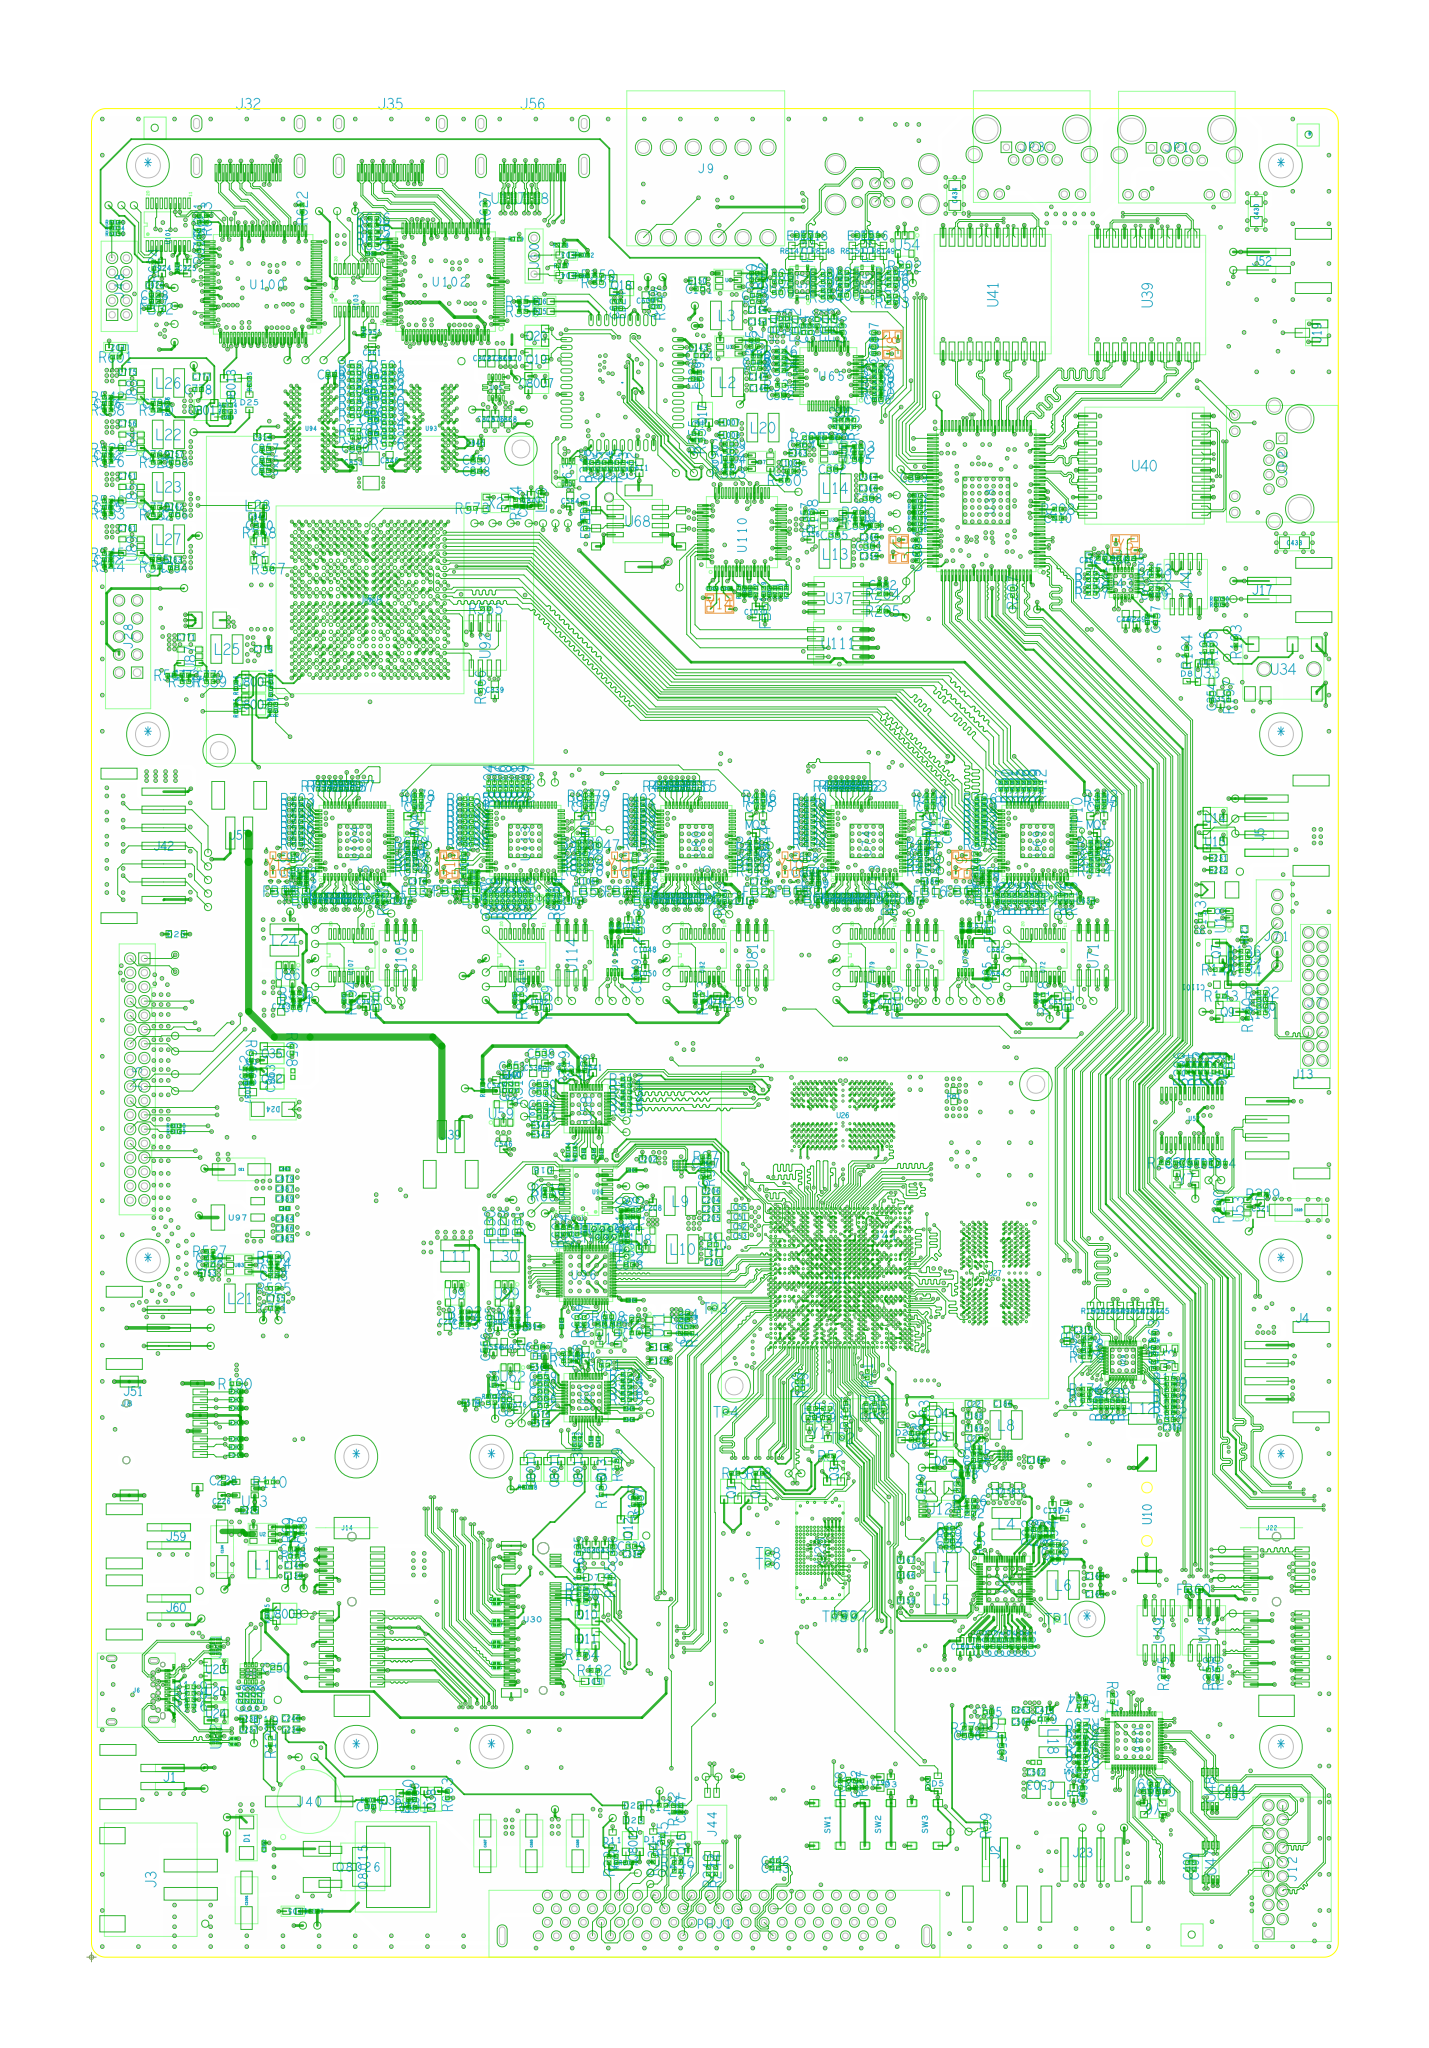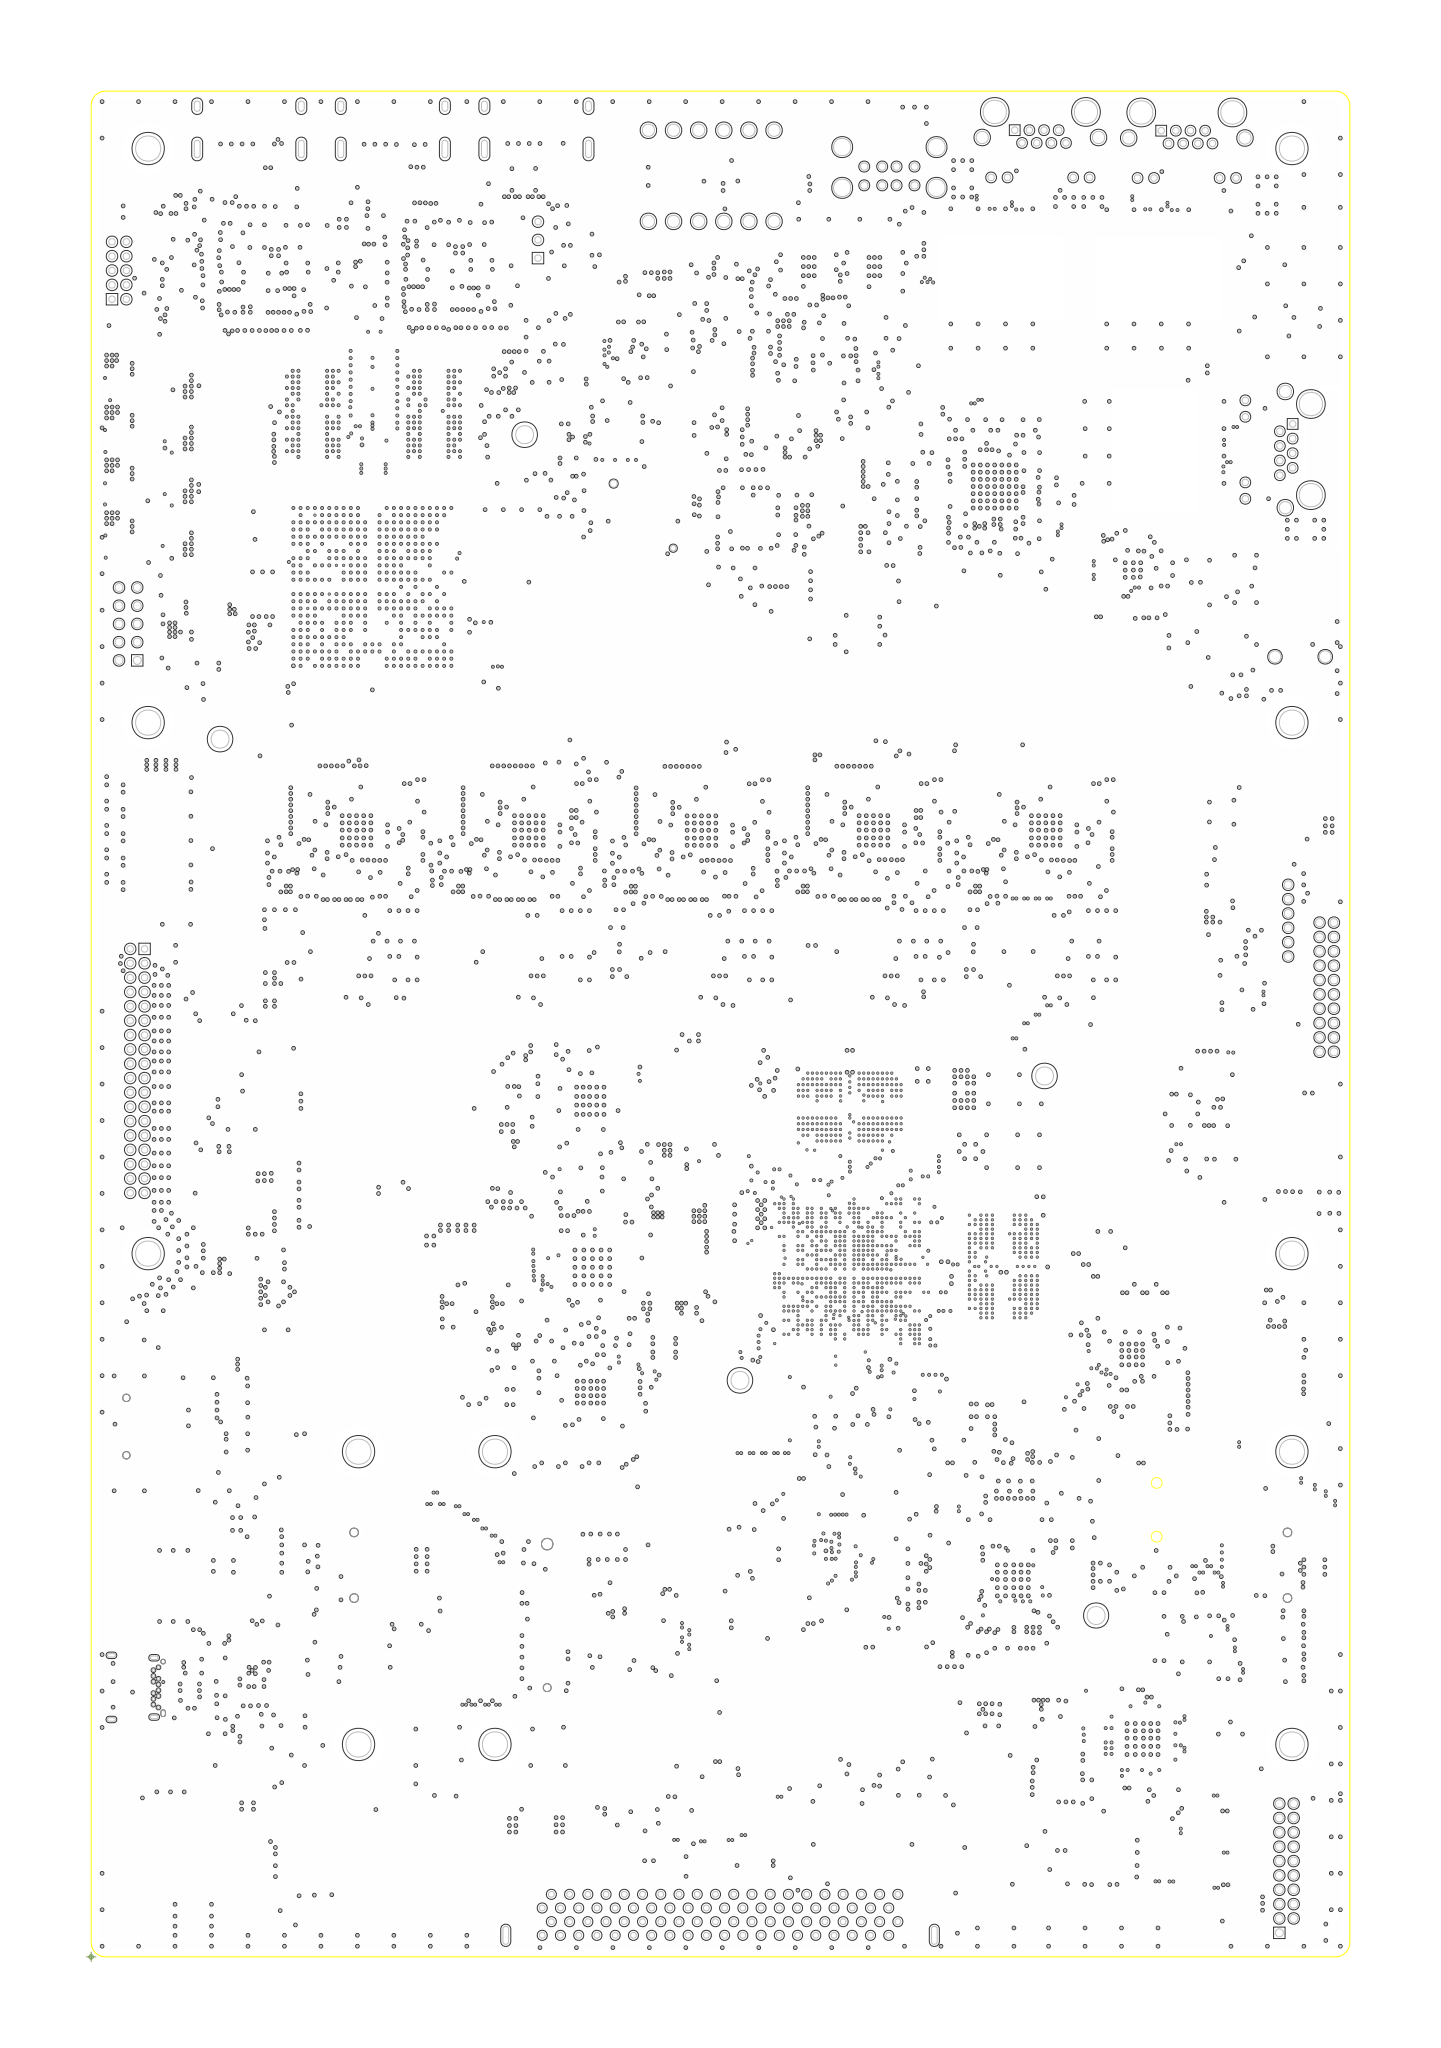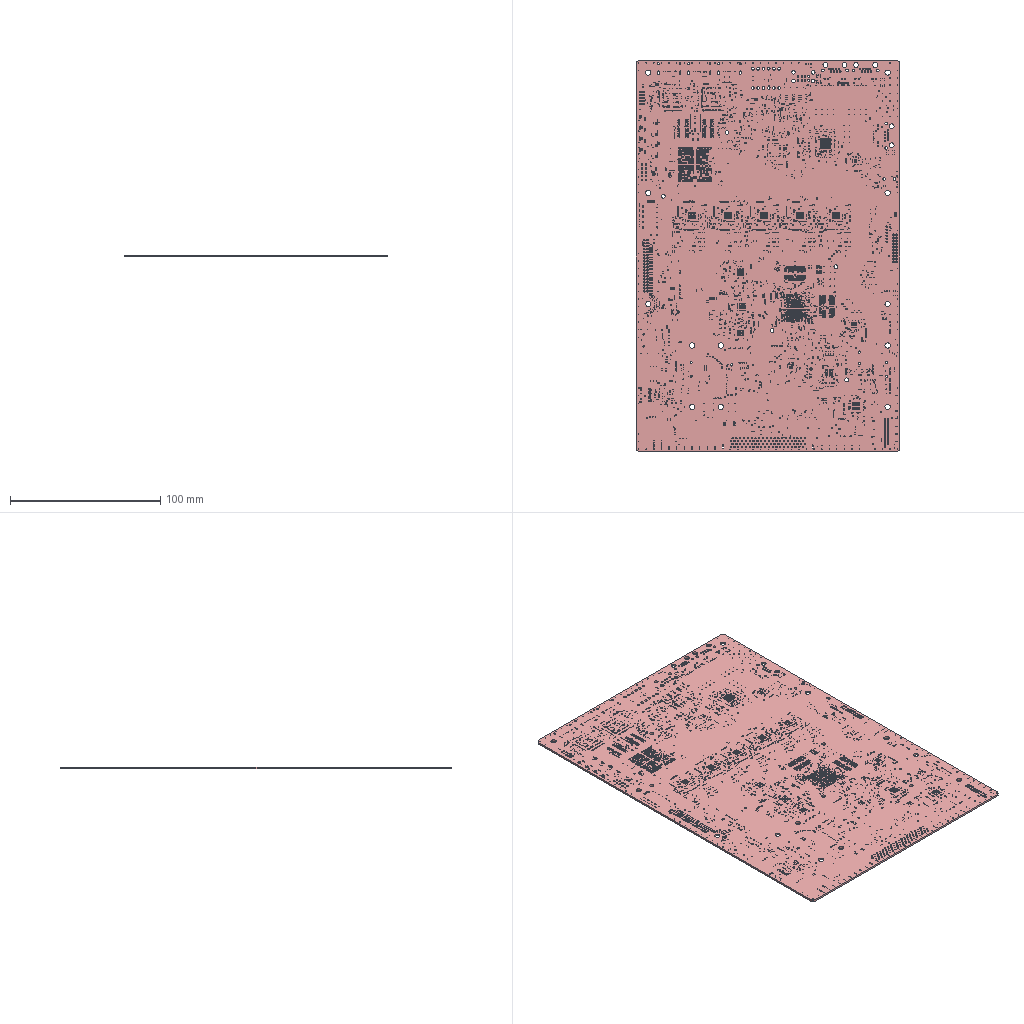Circuit board layout | Cadence Allegro | box 175.3 x 260 x 1.3 mm
Layer stack:
# Cadence Allegro layer stack of  (unit mm; from the constraint file cross-section; dielectric type: 0 not recorded (Allegro does not mark core vs prepreg), 3 surface material)
index,name,kind,layer,copper_thickness_mm,dielectric_type,dielectric_thickness_mm,dielectric_material,dielectric_constant
0,Top Surface,other,,,,,,
1,Dielectric1,dielectric,,,3,0.0249,FR-4,3.5
2,TOP,copper,TOP,0.0351,,,,
3,Dielectric2,dielectric,,,0,0.0749,FR-4,3.8
4,L2-GND,copper,L2-GND,0.017,,,,
5,Dielectric3,dielectric,,,0,0.2032,FR-4,4.5
6,L3,copper,L3,0.0305,,,,
7,Dielectric4,dielectric,,,0,0.2032,FR-4,4.5
8,L4-POWER,copper,L4-POWER,0.0305,,,,
9,Dielectric5,dielectric,,,0,0.1151,FR-4,3.8
10,L5-POWRE,copper,L5-POWRE,0.017,,,,
11,Dielectric6,dielectric,,,0,0.2032,FR-4,4.5
12,L6,copper,L6,0.0305,,,,
13,Dielectric7,dielectric,,,0,0.2032,FR-4,4.5
14,L7-GND,copper,L7-GND,0.0305,,,,
15,Dielectric8,dielectric,,,0,0.1151,FR-4,3.8
16,BOTTOM,copper,BOTTOM,0.0351,,,,
17,Dielectric9,dielectric,,,3,0.0249,FR-4,3.5
18,Bottom Surface,other,,,,,,
# drill layer pairs: low layer,high layer
drill_pair,TOP,BOTTOM
Part placement, first 572 of 2520 lines:
REFDES,COMP_VALUE,SYM_NAME,SYM_X,SYM_Y,SYM_ROTATE,SYM_MIRROR
C1,10uF,C0402,4153.838,3620.000,270.000,YES
C2,10uF,C0402,4352.539,3617.992,180.000,YES
C3,10uF,C0402,4150.000,3750.000,180.000,YES
C4,10uF,C0402,4155.807,3838.504,90.000,YES
C5,10uF,C0402,4345.767,3748.937,0.000,YES
C6,22uF,C0603,3440.000,3990.000,0.000,NO
C7,10uF,C0603,3445.000,3900.000,0.000,NO
C8,1uF,C0402,4010.744,3646.504,0.000,YES
C9,100nF,C0201,4077.744,3607.504,0.000,YES
C10,100nF,C0201,4077.744,3735.504,0.000,YES
C11,100nF,C0201,4075.497,3570.863,90.000,YES
C12,100nF,C0201,4077.744,3710.504,0.000,YES
C13,1nF,C0201,4077.744,3684.504,0.000,YES
C14,22uF,C0603,5554.744,2108.504,180.000,YES
C15,22uF,C0603,5554.744,2013.504,180.000,YES
C16,1uF,C0402,4158.744,3695.504,270.000,YES
C17,100nF,C0201,4108.744,3636.504,0.000,YES
C18,100nF,C0201,4111.744,3670.504,270.000,YES
C19,100nF,C0201,4209.744,3630.504,180.000,YES
C20,100nF,C0201,4206.744,3663.504,180.000,YES
C21,1nF,C0201,4195.744,3589.504,90.000,YES
C22,22uF,C0603,4884.744,3063.504,180.000,NO
C23,22uF,C0603,4884.744,2873.504,180.000,NO
C24,22uF,C0603,4884.744,2873.504,0.000,YES
C25,1uF,C0402,4514.744,3513.504,180.000,YES
C26,100nF,C0201,4272.744,3667.504,90.000,YES
C27,100nF,C0201,4285.744,3701.504,180.000,YES
C28,100nF,C0201,4259.744,3594.504,180.000,YES
C29,100nF,C0201,4246.744,3641.504,90.000,YES
C30,100nF,C0201,4297.744,3616.504,90.000,YES
C31,1nF,C0201,4297.744,3667.504,90.000,YES
C32,22uF,C0603,4443.208,3760.748,180.000,YES
C33,10uF,C0603,5130.000,2580.000,90.000,NO
C34,1uF,C0402,4250.000,3750.000,0.000,YES
C35,100nF,C0201,4262.744,3812.504,180.000,YES
C36,100nF,C0201,4211.744,3838.504,180.000,YES
C37,100nF,C0201,4211.744,3812.504,180.000,YES
C38,100nF,C0201,4262.744,3863.504,180.000,YES
C39,1nF,C0201,4211.744,3889.504,0.000,YES
C40,22uF,C0603,3588.681,4047.126,0.000,YES
C41,22uF,C0603,3588.681,3993.937,0.000,YES
C42,22uF,C0603,3589.744,4100.315,0.000,YES
C43,1uF,C0402,4154.822,3915.275,270.000,YES
C44,100nF,C0201,4051.744,3838.504,0.000,YES
C45,100nF,C0201,4103.744,3812.504,180.000,YES
C46,100nF,C0201,4103.744,3785.504,180.000,YES
C47,100nF,C0201,4051.744,3786.504,0.000,YES
C48,100nF,C0201,4081.744,3876.504,180.000,YES
C49,100nF,C0201,4051.744,3811.504,0.000,YES
C50,1nF,C0201,4077.744,3760.504,0.000,YES
C51,22uF,C0603,3589.744,4100.315,180.000,NO
C52,22uF,C0603,3588.681,4047.126,180.000,NO
C53,22uF,C0603,3588.681,3993.937,180.000,NO
C54,22uF,C0603,3589.744,4153.504,0.000,YES
C55,22uF,C0603,3589.744,4153.504,180.000,NO
C56,100nF,C0201,4109.744,3393.504,180.000,YES
C57,DNP,C0402,4174.744,3048.504,90.000,NO
C58,22pF,C0402,3984.744,2988.504,180.000,NO
C59,22pF,C0402,4064.744,2988.504,180.000,NO
C60,100nF,C0201,4387.539,3827.992,180.000,YES
C61,100nF,C0201,4052.539,3517.992,90.000,YES
C62,1uF,C0402,3977.539,3522.992,90.000,YES
C63,100nF,C0201,3947.539,3877.992,0.000,YES
C64,100nF,C0201,4362.539,3672.992,180.000,YES
C65,100nF,C0201,3912.539,3552.992,0.000,YES
C66,22uF,C0603,4678.744,3748.504,270.000,YES
C67,10uF,C0402,4378.646,3980.311,180.000,YES
C68,1uF,C0402,4091.744,4005.504,0.000,YES
C69,100nF,C0201,4118.539,3956.992,270.000,YES
C70,100nF,C0201,4226.744,3978.504,270.000,YES
C71,100nF,C0201,4093.539,3956.992,270.000,YES
C72,100nF,C0201,4201.744,3978.504,270.000,YES
C73,100nF,C0201,4272.744,3956.504,270.000,YES
C74,100nF,C0201,4145.744,3976.504,270.000,YES
C75,22uF,C0603,4159.744,4424.504,90.000,YES
C76,10uF,C0402,4432.539,3673.992,180.000,YES
C77,1uF,C0402,5202.744,4143.504,180.000,YES
C78,100nF,C0201,4288.539,3888.992,0.000,YES
C79,100nF,C0201,4339.744,3786.504,180.000,YES
C80,100nF,C0201,4312.744,3922.504,180.000,YES
C81,100nF,C0201,4336.744,3875.504,180.000,YES
C82,100nF,C0201,4338.744,3850.504,180.000,YES
C83,100nF,C0201,4309.744,3825.504,0.000,YES
C84,100nF,C0201,4297.744,3956.504,270.000,YES
C85,100nF,C0201,4232.744,4017.504,0.000,YES
C86,100nF,C0201,4148.744,3525.504,180.000,YES
C87,100nF,C0201,4340.744,3710.504,180.000,YES
C88,100nF,C0201,4390.744,3854.504,180.000,YES
C89,100nF,C0201,4169.539,3980.992,270.000,YES
C90,100nF,C0201,4386.520,3645.666,180.000,YES
C91,100nF,C0201,3990.539,3956.992,90.000,YES
C92,100nF,C0201,4155.744,3559.504,90.000,YES
C93,100nF,C0201,4137.744,3491.504,90.000,YES
C94,100nF,C0201,4099.119,3570.863,270.000,YES
C95,100nF,C0201,4077.744,3483.504,0.000,YES
C96,100nF,C0201,3957.000,3701.000,270.000,YES
C97,100nF,C0201,4209.355,3716.532,180.000,YES
C98,100nF,C0201,4204.744,3687.504,0.000,YES
C99,100nF,C0201,3916.744,3622.504,270.000,YES
C100,100nF,C0201,3812.744,3434.504,90.000,YES
C101,100nF,C0201,4209.744,3546.504,270.000,YES
C102,10nF,C0402,4229.586,958.561,270.000,NO
C103,100nF,C0201,3947.539,3827.992,0.000,YES
C104,100nF,C0201,4364.744,3523.504,180.000,YES
C105,100nF,C0201,3922.539,3927.992,0.000,YES
C106,100nF,C0201,3945.576,3799.209,0.000,YES
C107,100nF,C0201,4704.744,3378.504,180.000,YES
C108,100nF,C0201,4704.744,3353.504,180.000,YES
C109,100nF,C0201,4704.744,3328.504,180.000,YES
C110,100nF,C0201,4704.744,3303.504,180.000,YES
C115,100nF,C0201,4704.744,3428.504,180.000,YES
C116,100nF,C0201,4704.744,3403.504,180.000,YES
C117,100nF,C0201,3139.744,3378.504,0.000,YES
C118,4.7uF,C0603,3139.744,3378.504,180.000,NO
C119,100nF,C0201,3139.744,3303.504,0.000,YES
C120,4.7uF,C0603,3139.744,3303.504,180.000,NO
C121,100nF,C0201,4002.808,3681.086,0.000,YES
C122,100nF,C0201,3920.744,3674.504,0.000,YES
C123,100nF,C0201,4022.000,3600.000,180.000,YES
C124,DNP,C0402,4379.744,3393.504,90.000,YES
C125,100nF,C0201,4313.744,3570.504,0.000,YES
C126,100nF,C0201,4241.744,3542.504,90.000,YES
C127,100nF,C0201,3979.744,4008.504,270.000,YES
C128,100nF,C0201,4015.744,3956.504,90.000,YES
C129,100nF,C0201,3854.744,3973.504,90.000,YES
C130,100nF,C0201,3980.744,3923.504,180.000,YES
C131,100nF,C0201,4055.744,4046.504,270.000,YES
C132,100nF,C0201,4303.843,3511.808,90.000,YES
C133,100nF,C0201,3912.744,3526.504,0.000,YES
C134,100uF/35V,ECAP_6D3X7D7,723.148,2258.981,180.000,NO
C135,100nF,C0402,950.000,2305.000,0.000,YES
C136,10uF,C0603,680.000,2245.000,90.000,YES
C137,100nF,C0402,770.000,2250.000,90.000,YES
C138,100pF,C0402,1165.000,2365.000,90.000,NO
C139,22uF,C0603,1117.700,2112.319,0.000,NO
C140,10uF,C0603,1120.000,2170.000,0.000,NO
C141,100nF,C0402,1120.000,2260.000,0.000,NO
C142,100nF,C0402,3529.744,8878.504,0.000,YES
C143,10uF,C0603,3359.744,8913.504,180.000,NO
C144,100nF,C0402,3364.744,8868.504,180.000,NO
C145,100pF,C0402,3680.965,8866.888,0.000,NO
C146,22uF,C0603,3693.828,8688.568,0.000,NO
C147,10uF,C0603,3690.965,8751.888,0.000,NO
C148,100nF,C0402,3680.965,8831.888,0.000,NO
C149,100nF,C0402,3524.744,9248.504,0.000,YES
C150,10uF,C0603,3354.744,9283.504,180.000,NO
C151,100nF,C0402,3364.744,9238.504,180.000,NO
C152,100pF,C0402,3717.230,9307.072,90.000,NO
C153,22uF,C0603,3685.965,9056.889,0.000,NO
C154,10uF,C0603,3685.965,9121.888,0.000,NO
C155,100nF,C0402,3675.965,9201.888,0.000,NO
C156,10uF,C0603,4864.744,2098.504,90.000,YES
C157,22uF,C0603,5000.000,2580.000,90.000,NO
C158,22uF,C0603,5065.000,2580.000,90.000,NO
C159,22uF,C0603,4508.744,1975.504,180.000,NO
C160,22uF,C0603,5255.139,2063.284,90.000,YES
C161,22uF,C0603,5089.964,2208.899,180.000,YES
C162,22uF,C0603,5553.744,2110.504,0.000,NO
C163,22uF,C0603,5553.744,2010.504,0.000,NO
C164,47pF,C0402,4748.744,2305.504,180.000,NO
C165,2.2uF,C0402,4540.000,2882.280,90.000,NO
C166,10uF,C0603,4508.744,2115.504,180.000,NO
C167,22uF,C0603,4508.744,2200.504,180.000,NO
C168,100nF,C0402,5213.744,2350.504,90.000,NO
C169,1uF,C0402,4913.744,2135.504,270.000,YES
C170,100nF,C0402,5334.744,2243.504,0.000,NO
C171,1uF,C0402,4979.744,2208.504,180.000,YES
C172,2.2uF,C0402,5334.744,2283.504,0.000,NO
C173,4.7uF,C0603,4863.744,1720.504,270.000,NO
C174,1uF,C0402,5191.744,2130.504,270.000,YES
C175,2.2uF,C0402,4909.744,1738.504,270.000,NO
C176,2.2uF,C0402,5129.744,1738.504,270.000,NO
C177,1uF,C0402,4958.744,1925.504,180.000,YES
C178,100nF,C0402,5164.744,1738.504,270.000,NO
C179,1uF,C0402,5191.744,2006.504,270.000,YES
C180,4.7uF,C0603,4808.744,1720.504,270.000,NO
C181,2.2uF,C0402,5199.744,1738.504,270.000,NO
C182,100nF,C0402,4900.415,2785.952,180.000,NO
C183,1uF,C0402,5128.744,1925.504,180.000,YES
C184,10uF,C0603,5229.744,2753.504,0.000,NO
C185,100nF,C0402,4989.744,1738.504,270.000,NO
C186,22uF,C0603,5045.000,3065.000,0.000,NO
C187,1uF,C0402,5024.744,1738.504,90.000,NO
C188,22uF,C0603,4884.744,2998.504,180.000,NO
C189,22uF,C0603,4884.744,2928.504,180.000,NO
C190,22uF,C0603,4884.744,2928.504,0.000,YES
C191,1uF,C0402,5043.744,1925.504,180.000,YES
C192,2.2uF,C0402,5094.744,1738.504,270.000,NO
C193,DNP,C0603,4366.862,967.246,90.000,NO
C194,1uF,C0402,4913.744,2010.504,270.000,YES
C195,1uF,C0402,5059.744,1738.504,270.000,NO
C196,100nF,C0402,4900.414,2750.952,180.000,NO
C197,10uF,C0603,5319.744,2473.504,270.000,NO
C198,100nF,C0402,4954.744,1738.504,90.000,NO
C199,100nF,C0402,4914.744,2213.504,270.000,YES
C200,10nF,C0402,5249.744,2348.504,90.000,NO
C201,100nF,C0402,3384.744,4338.504,270.000,NO
C202,10uF,C0603,3079.744,4418.504,180.000,NO
C203,22uF,C0603,3429.744,4143.504,0.000,NO
C204,22uF,C0603,3429.744,4193.504,0.000,NO
C205,22uF,C0603,3429.744,4093.504,0.000,NO
C206,22uF,C0603,3429.744,4243.504,0.000,NO
C207,100nF,C0402,3400.175,4397.267,0.000,NO
C208,10uF,C0603,3106.995,4149.602,90.000,NO
C209,22uF,C0603,3445.000,3850.000,0.000,NO
C210,100nF,C0402,3440.000,3945.000,0.000,NO
C211,DNP,C0402,2965.263,3980.311,90.000,NO
C212,10uF,C0603,1972.437,3519.678,270.000,NO
C213,100pF,C0402,2066.925,3503.930,180.000,NO
C214,10uF,C0603,1945.000,3905.000,0.000,YES
C215,100nF,C0402,1945.000,3955.000,0.000,YES
C216,22pF,C0402,2965.263,4118.106,270.000,NO
C217,100nF,C0402,2031.492,3720.465,0.000,YES
C218,1uF,C0402,4832.280,2675.000,0.000,NO
C219,22pF,C0402,4590.000,2600.000,270.000,NO
C220,22pF,C0402,3260.538,3472.438,270.000,NO
C221,22pF,C0402,4797.696,2601.237,270.000,NO
C222,100nF,C0402,4864.744,2458.504,0.000,NO
C223,2.2uF,C0402,3280.223,3531.493,0.000,NO
C224,100nF,C0402,3280.223,3562.989,0.000,NO
C225,4.7uF,C0603,875.000,2475.000,180.000,NO
C226,4.7uF,C0603,720.000,2525.000,270.000,NO
C227,2.2uF,C0402,3008.570,3531.493,180.000,NO
C228,100nF,C0402,730.000,2640.000,90.000,NO
C229,4.7uF,C0603,6429.744,3523.504,270.000,YES
C230,22uF,C0603,6504.349,3523.724,270.000,YES
C231,4.7uF,C0603,6237.684,6086.594,180.000,NO
C232,22uF,C0603,6237.464,6020.060,180.000,NO
C233,150uF,C3528,6246.019,5909.992,180.000,NO
C234,10uF,C0603,6381.528,5663.051,90.000,NO
C235,100nF,C0201,643.576,1522.989,90.000,YES
C236,100nF,C0201,268.418,1440.946,180.000,YES
C237,10uF,C0603,870.000,1260.000,180.000,NO
C238,22uF,C0603,870.000,1320.000,180.000,NO
C239,4.7uF,C0603,1105.000,1260.000,0.000,NO
C240,22uF,C0603,1104.663,1322.515,0.000,NO
C241,100nF,C0201,541.744,1589.504,0.000,YES
C242,100nF,C0201,541.744,1614.504,0.000,YES
C243,100nF,C0201,787.859,1179.115,180.000,NO
C244,100nF,C0201,787.859,1210.115,180.000,NO
C245,220pF,C0402,825.576,1434.989,270.000,NO
C246,220pF,C0402,930.577,1434.989,270.000,NO
C247,100nF,C0402,3261.962,821.140,270.000,NO
C248,1uF,C0402,895.577,1434.989,270.000,NO
C249,100nF,C0402,860.576,1434.989,270.000,NO
C250,100nF,C0402,1021.576,1602.989,0.000,NO
C251,22uF,C0603,4559.744,4838.504,180.000,YES
C252,1uF,C0402,4379.744,4878.504,180.000,YES
C253,100nF,C0402,3844.744,4778.504,270.000,YES
C254,100nF,C0402,3939.744,4878.504,0.000,YES
C255,100nF,C0402,4229.744,4878.504,180.000,YES
C256,100nF,C0402,3844.744,4483.504,90.000,YES
C257,100nF,C0402,4219.744,4448.504,180.000,YES
C258,100nF,C0402,4294.744,4448.504,180.000,YES
C259,22uF,C0603,5001.244,3684.604,270.000,YES
C260,1uF,C0402,4788.644,3556.304,270.000,YES
C261,100nF,C0402,4966.358,3949.331,270.000,YES
C262,100nF,C0402,5202.578,4098.937,180.000,YES
C263,100nF,C0402,4789.193,3725.669,90.000,YES
C264,100nF,C0402,5214.389,3555.630,90.000,YES
C265,100nF,C0402,5119.901,4098.937,180.000,YES
C266,100nF,C0402,5216.344,3802.904,90.000,YES
C267,10uF,C0603,4819.744,4418.504,180.000,YES
C268,1uF,C0402,4474.744,4553.504,90.000,YES
C269,100nF,C0402,4089.744,4878.504,0.000,YES
C270,100nF,C0402,3944.744,4448.504,0.000,YES
C271,100nF,C0402,4369.744,4448.504,180.000,YES
C272,100nF,C0402,4094.744,4448.504,0.000,YES
C273,100nF,C0402,3844.744,4853.504,270.000,YES
C274,100nF,C0402,4474.744,4733.504,90.000,YES
C275,100nF,C0402,4474.744,4808.504,90.000,YES
C276,100nF,C0402,3844.744,4558.504,90.000,YES
C277,10uF,C0603,5000.844,3543.004,90.000,YES
C278,1uF,C0402,5214.389,3720.984,90.000,YES
C279,100nF,C0402,4966.358,4028.071,90.000,YES
C280,100nF,C0402,4887.618,4098.937,0.000,YES
C281,100nF,C0402,4804.941,4098.937,0.000,YES
C282,100nF,C0402,4788.244,3638.604,270.000,YES
C283,100nF,C0402,5037.224,4028.071,90.000,YES
C284,100nF,C0402,4789.193,3845.157,270.000,YES
C285,100nF,C0402,5029.144,3925.104,270.000,YES
C286,100nF,C0402,5214.389,3886.338,270.000,YES
C287,10uF,C0603,4159.744,4913.504,270.000,YES
C288,100nF,C0402,4014.744,4878.504,180.000,YES
C289,100nF,C0402,4019.744,4448.504,180.000,YES
C290,100nF,C0402,4304.744,4878.504,0.000,YES
C291,10uF,C0603,5222.263,3984.764,270.000,YES
C292,100nF,C0402,5214.389,3638.307,270.000,YES
C293,100nF,C0402,4790.844,3927.204,270.000,YES
C294,100nF,C0402,4941.944,3845.204,90.000,YES
C295,2.2uF,C0402,4232.744,2162.504,0.000,YES
C296,4.7uF,C0603,4159.744,2203.504,180.000,YES
C297,100nF,C0402,3989.744,2248.504,90.000,YES
C298,4.7uF,C0603,4102.744,2389.504,180.000,YES
C299,100nF,C0402,3987.744,2184.504,0.000,YES
C300,100nF,C0402,6480.000,5267.000,0.000,NO
C301,100nF,C0402,6480.000,5304.000,0.000,NO
C302,100nF,C0402,6707.012,6216.480,90.000,YES
C303,10uF,C0603,6710.949,5944.827,0.000,YES
C304,100nF,C0402,6718.823,5992.071,0.000,YES
C305,10uF,C0603,6712.656,5790.596,0.000,YES
C306,10uF,C0603,6712.656,5880.596,0.000,YES
C307,100nF,C0402,6717.656,5835.596,0.000,YES
C308,DNP,C0402,5698.314,3137.781,0.000,YES
C309,10uF,C0603,5981.779,2933.057,0.000,NO
C310,100nF,C0402,5969.967,2976.364,0.000,NO
C311,100nF,C0402,5803.625,3318.802,90.000,YES
C312,100nF,C0402,5619.574,3224.395,270.000,YES
C313,100nF,C0402,5733.626,3398.803,0.000,YES
C314,100nF,C0402,5648.627,3398.802,0.000,YES
C315,4.7uF,C0603,5694.378,3212.585,0.000,YES
C316,100nF,C0402,5792.802,3212.584,180.000,YES
C317,22pF,C0402,5878.626,3277.740,270.000,NO
C318,22pF,C0402,5878.626,3357.739,90.000,NO
C319,4.7uF,C0603,5489.744,3473.504,0.000,NO
C320,100nF,C0402,5509.744,3428.504,0.000,NO
C321,100nF,C0402,5618.627,3338.802,90.000,YES
C322,100nF,C0402,5803.626,3398.803,270.000,YES
C323,10nF,C0402,5508.626,3358.802,180.000,NO
C324,100nF,C0201,2241.740,1603.147,0.000,NO
C325,100nF,C0201,2241.740,1626.769,0.000,NO
C326,100nF,C0201,2241.740,1721.257,0.000,NO
C327,100nF,C0201,2241.740,1744.879,0.000,NO
C328,100nF,C0201,2241.740,1839.367,0.000,NO
C329,100nF,C0201,2241.740,1862.989,0.000,NO
C330,100nF,C0201,2241.740,1957.477,0.000,NO
C331,100nF,C0201,2241.740,1981.099,0.000,NO
C332,22uF,C0603,2739.611,2254.404,90.000,NO
C333,10uF,C0603,2841.973,2254.404,90.000,NO
C334,10uF,C0603,2790.792,2254.404,90.000,NO
C335,100nF,C0402,2696.304,2254.404,90.000,NO
C336,100nF,C0402,2885.280,2254.404,90.000,NO
C337,100nF,C0402,3031.490,2523.617,270.000,NO
C338,10uF,C0603,2992.120,2232.279,0.000,NO
C339,100nF,C0402,2988.183,2275.586,0.000,NO
C340,100nF,C0402,3493.562,9715.630,270.000,YES
C341,100nF,C0402,3098.562,9680.630,0.000,YES
C342,100nF,C0402,3098.562,9768.630,0.000,YES
C343,100nF,C0402,3098.562,9718.630,0.000,YES
C344,100nF,C0402,3098.562,9818.630,0.000,YES
C345,10uF,C0603,575.000,2960.000,270.000,YES
C346,100nF,C0402,505.000,2960.000,270.000,YES
C347,100nF,C0402,3972.000,9709.000,270.000,YES
C348,100nF,C0402,3563.562,9685.630,0.000,YES
C349,100nF,C0402,3561.000,9792.000,0.000,YES
C350,100nF,C0402,3563.562,9720.630,0.000,YES
C351,100nF,C0402,3558.562,9855.630,0.000,YES
C352,100nF,C0402,6430.844,6945.304,90.000,YES
C353,4.7uF,C0603,6249.744,6968.504,270.000,NO
C354,100nF,C0402,6199.744,6978.504,270.000,NO
C355,100nF,C0402,4111.358,7874.921,180.000,NO
C356,10uF,C0603,3981.358,7879.921,270.000,NO
C357,100nF,C0402,3951.358,7979.921,90.000,NO
C358,100pF,C0402,4246.358,7929.921,180.000,NO
C359,22uF,C0603,4304.964,7758.109,0.000,NO
C360,10uF,C0603,4304.744,7863.504,0.000,NO
C361,100nF,C0402,4304.744,7813.504,0.000,NO
C362,100nF,C0402,4101.358,8239.921,180.000,NO
C363,10uF,C0603,3909.744,8328.504,180.000,NO
C364,100nF,C0402,3929.744,8373.504,180.000,NO
C365,100pF,C0402,4241.358,8294.921,180.000,NO
C366,22uF,C0603,4300.126,8133.451,0.000,NO
C367,10uF,C0603,4299.906,8196.838,0.000,NO
C368,100nF,C0402,4299.906,8078.728,0.000,NO
C369,1uF,C0402,5250.442,8116.748,0.000,YES
C370,10nF,C0402,5250.442,8081.315,0.000,YES
C371,1uF,C0402,5218.169,7652.992,180.000,YES
C372,1uF,C0402,4769.744,8393.504,90.000,YES
C373,NC-10uF/10V-Y5V,C0603,4743.755,8476.201,0.000,YES
C374,10nF,C0402,4740.850,8255.893,180.000,YES
C375,10uF,C0603,4638.169,7892.992,0.000,YES
C376,NC-10uF/10V-Y5V,C0603,4642.425,8291.326,0.000,YES
C377,1uF,C0402,4634.744,8393.504,90.000,YES
C378,1uF,C0402,4669.744,8393.504,90.000,YES
C379,10uF,C0603,4588.169,8382.992,90.000,YES
C380,22pF,C0402,4570.649,7750.748,270.000,NO
C381,22pF,C0402,4570.649,7829.488,270.000,NO
C382,10nF,C0402,4379.744,7598.504,0.000,NO
C383,1uF,C0402,4751.319,7762.559,180.000,YES
C384,10nF,C0402,4803.169,7652.992,180.000,YES
C385,1uF,C0402,5067.027,7740.000,270.000,YES
C386,10nF,C0402,5098.523,7740.000,270.000,YES
C387,10nF,C0402,5074.744,8393.504,90.000,YES
C388,1uF,C0402,5109.744,8393.504,90.000,YES
C389,10nF,C0402,5035.531,8282.244,90.000,YES
C390,10nF,C0402,4979.744,7743.504,270.000,YES
C391,10nF,C0402,4994.744,8393.504,90.000,YES
C392,10nF,C0402,5159.744,8253.504,0.000,YES
C393,10nF,C0402,5155.452,8034.212,0.000,YES
C394,10nF,C0402,5218.169,7687.991,180.000,YES
C395,10nF,C0402,5159.744,7863.504,0.000,YES
C396,10nF,C0402,5199.744,8393.504,90.000,YES
C397,10nF,C0402,5159.744,7898.504,0.000,YES
C398,10nF,C0402,4804.744,8393.504,90.000,YES
C399,10nF,C0402,4553.169,8192.991,180.000,NO
C400,10nF,C0402,4748.022,7917.307,180.000,YES
C401,10nF,C0402,4748.169,7852.992,180.000,YES
C402,10nF,C0402,4740.850,8216.523,180.000,YES
C403,10nF,C0402,4740.850,8177.153,180.000,YES
C404,10nF,C0402,4748.169,7812.992,180.000,YES
C405,10nF,C0402,4884.744,7743.504,270.000,YES
C406,10nF,C0402,4751.319,7703.504,180.000,YES
C407,10nF,C0402,5159.744,7783.504,0.000,YES
C408,10nF,C0402,5159.744,8153.504,0.000,YES
C409,10nF,C0402,5155.452,8065.709,0.000,YES
C410,10nF,C0402,5349.744,7968.504,0.000,NO
C411,10nF,C0402,5149.744,8338.504,0.000,YES
C412,10nF,C0402,4904.744,8393.504,90.000,YES
C413,10nF,C0402,4704.744,8393.504,90.000,YES
C414,1nF/1KV,C1206,5492.539,9552.992,270.000,YES
C415,NC-0.01uF/25V-X7R,C0402,5568.394,8893.674,270.000,YES
C416,NC-0.01uF/25V-X7R,C0402,5718.001,8893.675,270.000,YES
C417,10nF,C0402,5867.606,8893.674,270.000,YES
C418,NC-0.01uF/25V-X7R,C0402,6017.212,8893.675,270.000,YES
C419,NC-0.01uF/25V-X7R,C0402,5513.838,8533.972,180.000,YES
C420,NC-0.01uF/25V-X7R,C0402,5513.838,8384.373,180.000,YES
C421,10nF,C0402,5513.838,8233.972,180.000,YES
C422,NC-0.01uF/25V-X7R,C0402,5513.838,8084.374,180.000,YES
C423,1nF/1KV,C1206,6182.972,8630.118,180.000,YES
C424,NC-0.01uF/25V-X7R,C0402,4713.685,8893.858,270.000,YES
C425,NC-0.01uF/25V-X7R,C0402,4863.284,8893.858,270.000,YES
C426,10nF,C0402,5013.685,8893.858,270.000,YES
C427,NC-0.01uF/25V-X7R,C0402,5163.283,8893.858,270.000,YES
C428,1nF/1KV,C1206,5337.539,9552.992,270.000,YES
C429,1nF/1KV,C1206,6448.044,9666.004,270.000,YES
C430,1nF/1KV,C1206,6448.044,9666.004,90.000,NO
C431,1nF/1KV,C1206,6658.900,7832.400,180.000,YES
C432,1nF/1KV,C1206,4778.696,9755.144,270.000,YES
C433,1nF/1KV,C1206,6658.900,7832.400,0.000,NO
C434,1nF/1KV,C1206,4778.696,9755.144,90.000,NO
C435,100uF,ECAP_6D3X7D7,2435.098,629.921,0.000,NO
C436,100uF,ECAP_6D3X7D7,2691.004,629.921,0.000,NO
C437,100uF,ECAP_6D3X7D7,2179.193,629.921,0.000,NO
C442,100nF,C0402,3784.744,533.504,0.000,NO
C443,100nF,C0402,3784.744,493.504,0.000,NO
C445,22pF,C0402,5751.744,7744.504,0.000,NO
C446,22pF,C0402,5669.744,7744.504,180.000,NO
C447,4.7uF,C0603,5724.744,7408.504,270.000,NO
C448,100nF,C0402,5767.744,7538.504,180.000,YES
C449,100nF,C0402,5884.744,7543.504,0.000,NO
C450,100nF,C0402,5642.539,7637.992,90.000,YES
C451,100nF,C0402,5767.744,7486.504,180.000,YES
C452,4.7uF,C0603,5519.744,7736.504,90.000,NO
C453,100nF,C0402,5799.744,7618.504,0.000,YES
C454,100nF,C0402,5687.744,7538.504,0.000,YES
C455,100nF,C0402,5697.539,7682.992,180.000,YES
C456,1uF,C0402,5631.744,7736.504,270.000,YES
C457,100nF,C0402,5889.744,7408.504,270.000,NO
C458,1uF,C0402,5844.744,7408.504,270.000,NO
C459,10uF,C0603,5403.000,887.500,0.000,YES
C460,10uF,C0603,5373.200,1105.000,90.000,YES
C461,NC/100P,C0402,5890.000,1330.000,270.000,YES
C462,100nF,C0402,5635.000,1315.000,0.000,YES
C463,100nF,C0402,5866.844,1072.461,90.000,YES
C466,100nF,C0402,5635.000,1200.000,0.000,YES
C467,100nF,C0402,5930.000,1330.000,90.000,YES
C468,100nF,C0402,5897.539,1130.000,180.000,YES
C469,100nF,C0402,5795.256,1071.496,90.000,YES
C470,100nF,C0402,5830.256,1071.496,90.000,YES
C471,100nF,C0402,5906.842,1072.461,90.000,YES
C472,100nF,C0402,5900.000,1205.000,180.000,YES
C473,100nF,C0402,5740.000,1070.000,90.000,YES
C476,100nF,C0402,6156.744,1806.504,0.000,YES
C477,22pF,C0402,6156.744,1841.504,0.000,YES
C478,10uF,C0603,5274.744,1368.504,180.000,NO
C479,NC/100P,C0402,5269.744,1318.504,180.000,NO
C480,100nF,C0402,5700.000,1070.000,90.000,YES
C481,100nF,C0402,5635.000,1270.000,0.000,YES
C482,10nF,C0402,5897.539,1166.842,180.000,YES
C483,100nF,C0402,5900.000,1245.000,180.000,YES
C484,100nF,C0402,5780.000,1330.000,270.000,YES
C485,100nF,C0402,5635.000,1235.000,0.000,YES
C486,100nF,C0402,6350.000,185.000,90.000,YES
C488,100nF,C0402,5635.000,1165.000,0.000,YES
C490,100nF,C0402,6068.504,505.256,270.000,NO
C491,100nF,C0402,6103.504,505.256,270.000,NO
C492,1uF,C0402,5483.539,1183.843,0.000,NO
C493,100nF,C0402,6310.000,895.000,0.000,NO
C494,100nF,C0402,6310.000,930.000,0.000,NO
C495,100nF,C0402,6382.000,1014.000,90.000,YES
C496,12p,C0402,5922.539,916.843,180.000,NO
C497,12p,C0402,5842.540,916.843,0.000,NO
C498,100nF,C0402,5486.842,919.462,90.000,NO
C499,100nF,C0402,5857.504,1958.256,0.000,YES
C500,10uF,C0603,5515.000,1195.000,90.000,YES
C501,104,C0402,5635.000,1355.000,180.000,YES
C502,22uF,C0603,5229.000,1024.000,180.000,NO
C503,100nF,C0402,5229.000,1079.000,180.000,NO
C504,2.2nF,C0402,5484.412,1430.000,180.000,NO
C505,1uF,C0402,4964.744,1358.504,0.000,NO
C506,NC,C0402,4849.744,1228.504,0.000,NO
C507,NC,C0402,5039.118,1153.771,90.000,NO
C508,4.7uF,C0603,5144.744,1303.504,180.000,NO
C509,22pF,C0402,6018.917,4397.693,180.000,NO
C510,100nF,C0402,6027.547,4783.455,270.000,YES
C511,22pF,C0402,6098.917,4397.694,0.000,NO
C512,10uF,C0603,6070.854,4767.707,270.000,YES
C513,100nF,C0402,5994.721,4606.837,90.000,YES
C514,100nF,C0402,6030.154,4606.837,90.000,YES
C515,100nF,C0402,5923.855,4606.837,90.000,YES
C516,100nF,C0402,5959.288,4606.837,90.000,YES
C517,100nF,C0402,6165.342,4755.896,90.000,YES
C518,100nF,C0402,6156.138,4606.837,90.000,YES
C519,1uF,C0402,6230.744,4606.496,90.000,YES
C520,100uF,ECAP_6D3X7D7,6681.089,4137.787,270.000,NO
C521,10uF,C0603,6472.620,4145.551,270.000,NO
C522,10uF,C0402,4292.539,9182.992,0.000,YES
C523,10uF,C0402,4541.000,9523.000,270.000,YES
C524,10uF,C0402,3922.971,9182.992,0.000,YES
C525,10uF,C0402,3330.000,9033.000,180.000,YES
C526,100nF,C0402,2730.779,4926.922,90.000,NO
C527,10uF,C0603,2445.000,4925.000,270.000,YES
C528,100nF,C0402,2619.744,4736.504,90.000,YES
C529,100nF,C0402,2619.744,4814.504,270.000,YES
C530,100nF,C0402,2495.779,4831.922,180.000,NO
C531,2.2uF,C0402,2821.922,4447.221,270.000,NO
C532,2.2uF,C0402,2856.000,4626.000,90.000,YES
C533,105,C0402,2495.000,4790.000,0.000,NO
C534,105,C0402,2495.000,4720.000,0.000,NO
C535,2.2uF,C0402,2725.106,4448.814,270.000,NO
C536,2.2uF,C0402,2780.224,4448.814,270.000,NO
C537,105,C0402,2495.779,4686.922,0.000,NO
C538,100nF,C0402,2487.925,5004.061,180.000,NO
C539,10uF,C0603,2445.000,4925.000,90.000,NO
C540,100nF,C0402,2701.484,4814.955,180.000,YES
C541,10uF,C0603,2775.779,4926.922,90.000,NO
C542,100nF,C0402,2780.224,4814.955,180.000,YES
C543,105,C0402,2495.779,4651.922,0.000,NO
C544,4.7uF,C0603,2485.779,4606.922,180.000,NO
C545,4.7uF,C0603,2485.779,4556.922,180.000,NO
C546,10uF,C0603,2280.225,4503.932,270.000,NO
C547,10uF,C0603,2240.779,4826.922,90.000,NO
C548,100nF,C0402,2285.779,4816.922,90.000,NO
C549,100nF,C0402,2320.779,4816.922,90.000,NO
C550,10uF,C0603,2325.779,4886.922,180.000,NO
C551,100nF,C0402,2331.406,4933.065,180.000,NO
C552,100nF,C0402,2320.000,4705.000,90.000,YES
C553,100nF,C0402,2689.744,3318.504,90.000,NO
C554,10uF,C0603,2224.744,3378.504,270.000,NO
C555,100nF,C0402,2179.744,3378.504,90.000,YES
C556,100nF,C0402,2179.744,3378.504,270.000,NO
C558,2.2uF,C0402,2765.000,2855.000,270.000,NO
C559,100nF,C0402,2500.000,3215.000,180.000,NO
C560,105,C0402,2500.000,3175.000,0.000,NO
C561,105,C0402,2500.000,3135.000,0.000,NO
C563,2.2uF,C0402,2804.744,2853.504,270.000,NO
C564,2.2uF,C0402,2975.779,2976.922,0.000,NO
C565,2.2uF,C0402,2975.779,3036.922,0.000,NO
C566,105,C0402,2500.000,3095.000,0.000,NO
C567,100nF,C0402,2479.744,3378.504,0.000,NO
C568,10uF,C0603,2479.744,3268.504,180.000,NO
C569,100nF,C0402,2664.744,3218.504,0.000,YES
C570,10uF,C0603,2734.744,3333.504,90.000,NO
C571,100nF,C0402,2764.744,3218.504,180.000,YES
C572,105,C0402,2500.000,3055.000,0.000,NO
C573,4.7uF,C0603,2485.779,3006.922,180.000,NO
C574,4.7uF,C0603,2485.779,2956.922,180.000,NO
C575,10uF,C0603,2378.709,3380.086,90.000,NO
C576,10uF,C0603,2358.709,3060.086,270.000,NO
C577,100nF,C0402,2313.709,3070.086,270.000,NO
C578,100nF,C0402,2278.709,3070.086,270.000,NO
C579,10uF,C0603,2100.000,3070.000,180.000,NO
C580,100nF,C0402,2100.000,3070.000,0.000,YES
C581,100nF,C0402,2228.709,3185.086,90.000,NO
C582,100nF,C0402,3207.234,8814.105,0.000,YES
C583,100nF,C0402,3207.234,8849.538,0.000,YES
C584,NC/10uF,C0603,2649.744,8063.504,270.000,NO
C585,NC/10uF,C0603,2614.744,8243.504,90.000,YES
C586,100nF,C0402,2829.282,8471.586,270.000,YES
C587,NC/10uF,C0603,3207.234,8711.743,180.000,YES
C588,NC/10uF,C0603,2785.974,8471.586,90.000,YES
Pad and via stacks, first 107 of 228 lines:
# Allegro (Cadence) via spans and padstacks; design units: ("mils" 3 1000)
# via spans: padstack,start_layer,end_layer,net_example,count
VIA6-12,ETCH/TOP,ETCH/BOTTOM,VCC_3V3_FPGA,893
VIA8-16,ETCH/TOP,ETCH/BOTTOM,VCC_3V3_FPGA,977
VIA20D10,ETCH/TOP,ETCH/BOTTOM,DGND,3870
# Allegro padstack definitions: name,start_layer,end_layer,drill,plating,holeType,type
S_C0R325,"ETCH/TOP","ETCH/TOP",0.0,"NON_PLATED","none","smd"
S_R0R80X1R10,"ETCH/TOP","ETCH/TOP",0.0,"NON_PLATED","none","smd"
S_C0R70,"ETCH/TOP","ETCH/TOP",0.0,"NON_PLATED","none","smd"
S_R0R20X0R68,"ETCH/TOP","ETCH/TOP",0.0,"NON_PLATED","none","smd"
S_R0R40X0R75,"ETCH/TOP","ETCH/TOP",0.0,"NON_PLATED","none","smd"
S_R1R40X1R20,"ETCH/TOP","ETCH/TOP",0.0,"NON_PLATED","none","smd"
S_R0R65X0R80,"ETCH/TOP","ETCH/TOP",0.0,"NON_PLATED","none","smd"
S_S0R50,"ETCH/TOP","ETCH/TOP",0.0,"PLATED","none","smd"
S_R0R80X0R90,"ETCH/TOP","ETCH/TOP",0.0,"PLATED","none","smd"
S_R0R95X1R30,"ETCH/TOP","ETCH/TOP",0.0,"PLATED","none","smd"
S_S0R55,"ETCH/TOP","ETCH/TOP",0.0,"PLATED","none","smd"
S_R0R25X0R30,"ETCH/TOP","ETCH/TOP",0.0,"NON_PLATED","none","smd"
S_R0R30X2R60,"ETCH/TOP","ETCH/TOP",0.0,"NON_PLATED","none","smd"
S_R0R70X0R90,"ETCH/TOP","ETCH/TOP",0.0,"NON_PLATED","none","smd"
SR0R76X1R50,"ETCH/TOP","ETCH/TOP",0.0,"PLATED","none","smd"
S_C0R30,"ETCH/TOP","ETCH/TOP",0.0,"NON_PLATED","none","smd"
S_R0R50X2R00,"ETCH/TOP","ETCH/TOP",0.0,"NON_PLATED","none","smd"
S_R0R50X0R30,"ETCH/TOP","ETCH/TOP",0.0,"NON_PLATED","none","smd"
S_R0R30X0R70,"ETCH/TOP","ETCH/TOP",0.0,"NON_PLATED","none","smd"
S_R0R60X0R30,"ETCH/TOP","ETCH/TOP",0.0,"NON_PLATED","none","smd"
S_R0R30X0R60,"ETCH/TOP","ETCH/TOP",0.0,"NON_PLATED","none","smd"
S_S1R45,"ETCH/TOP","ETCH/TOP",0.0,"PLATED","none","smd"
S_R0R70X2R00,"ETCH/TOP","ETCH/TOP",0.0,"NON_PLATED","none","smd"
S_S1R00,"ETCH/TOP","ETCH/TOP",0.0,"NON_PLATED","none","smd"
S_R0R80X0R60,"ETCH/TOP","ETCH/TOP",0.0,"NON_PLATED","none","smd"
S_C0R20,"ETCH/TOP","ETCH/TOP",0.0,"NON_PLATED","none","smd"
S_R1R00X1R20,"ETCH/TOP","ETCH/TOP",0.0,"NON_PLATED","none","smd"
S_C1R00,"ETCH/TOP","ETCH/TOP",0.0,"NON_PLATED","none","smd"
S_R0R30X1R45,"ETCH/TOP","ETCH/TOP",0.0,"NON_PLATED","none","smd"
S_O0R30X1R45,"ETCH/TOP","ETCH/TOP",0.0,"NON_PLATED","none","smd"
S_C0R50,"ETCH/TOP","ETCH/TOP",0.0,"NON_PLATED","none","smd"
S_C0R24,"ETCH/TOP","ETCH/TOP",0.0,"NON_PLATED","none","smd"
R85X42,"ETCH/TOP","ETCH/TOP",0.0,"NON_PLATED","none","smd"
SMD_R160X50,"ETCH/TOP","ETCH/TOP",0.0,"NON_PLATED","none","smd"
S_R0R80X2R90,"ETCH/TOP","ETCH/TOP",0.0,"NON_PLATED","none","smd"
S_R0R80X2R60,"ETCH/TOP","ETCH/TOP",0.0,"NON_PLATED","none","smd"
SHAPEESD0402_L,"ETCH/TOP","ETCH/TOP",0.0,"PLATED","none","smd"
SHAPEESD0402_R,"ETCH/TOP","ETCH/TOP",0.0,"PLATED","none","smd"
S_R0R965X0R80,"ETCH/TOP","ETCH/TOP",0.0,"NON_PLATED","none","smd"
S_R3R00X5R00,"ETCH/TOP","ETCH/TOP",0.0,"PLATED","none","smd"
R60X160,"ETCH/TOP","ETCH/TOP",0.0,"NON_PLATED","none","smd"
S_R3R40X1R30,"ETCH/TOP","ETCH/TOP",0.0,"NON_PLATED","none","smd"
S_O0R70X1R00,"ETCH/TOP","ETCH/TOP",0.0,"NON_PLATED","none","smd"
S_R0R70X1R00,"ETCH/TOP","ETCH/TOP",0.0,"NON_PLATED","none","smd"
S_O0R80X0R15,"ETCH/TOP","ETCH/TOP",0.0,"NON_PLATED","none","smd"
S_R0R80X0R15,"ETCH/TOP","ETCH/TOP",0.0,"NON_PLATED","none","smd"
S_R0R15X0R80,"ETCH/TOP","ETCH/TOP",0.0,"NON_PLATED","none","smd"
S_S5R00,"ETCH/TOP","ETCH/TOP",0.0,"NON_PLATED","none","smd"
SMDR145X105,"ETCH/TOP","ETCH/TOP",0.0,"PLATED","none","smd"
S_O1R10X0R60,"ETCH/TOP","ETCH/TOP",0.0,"NON_PLATED","none","smd"
S_R1R10X0R60,"ETCH/TOP","ETCH/TOP",0.0,"NON_PLATED","none","smd"
SMDR40X16,"ETCH/TOP","ETCH/TOP",0.0,"NON_PLATED","none","smd"
SMD_CIR0M3,"ETCH/TOP","ETCH/TOP",0.0,"NON_PLATED","none","smd"
SMD1M125X0M5,"ETCH/TOP","ETCH/TOP",0.0,"NON_PLATED","none","smd"
S_R0R65X0R25,"ETCH/TOP","ETCH/TOP",0.0,"NON_PLATED","none","smd"
S_R0R25X0R65,"ETCH/TOP","ETCH/TOP",0.0,"NON_PLATED","none","smd"
S_S3R50,"ETCH/TOP","ETCH/TOP",0.0,"NON_PLATED","none","smd"
S_R1R20X0R60,"ETCH/TOP","ETCH/TOP",0.0,"NON_PLATED","none","smd"
S_R1R20X1R50,"ETCH/TOP","ETCH/TOP",0.0,"NON_PLATED","none","smd"
R70X50,"ETCH/TOP","ETCH/TOP",0.0,"PLATED","none","smd"
R30X50,"ETCH/TOP","ETCH/TOP",0.0,"PLATED","none","smd"
R45X55,"ETCH/TOP","ETCH/TOP",0.0,"PLATED","none","smd"
R42X57,"ETCH/TOP","ETCH/TOP",0.0,"PLATED","none","smd"
SMD20_17,"ETCH/TOP","ETCH/TOP",0.0,"PLATED","none","smd"
SMD65REC13,"ETCH/TOP","ETCH/TOP",0.0,"PLATED","none","smd"
SMD0R8X0R8,"ETCH/TOP","ETCH/TOP",0.0,"PLATED","none","smd"
C28X28,"ETCH/TOP","ETCH/TOP",0.0,"PLATED","none","smd"
C14_17,"ETCH/TOP","ETCH/TOP",0.0,"NON_PLATED","none","smd"
OB11_03X33_47,"ETCH/TOP","ETCH/TOP",0.0,"PLATED","none","smd"
RE11,"ETCH/TOP","ETCH/TOP",0.0,"PLATED","none","smd"
C19_7,"ETCH/TOP","ETCH/TOP",0.0,"NON_PLATED","none","smd"
S20X20,"ETCH/TOP","ETCH/TOP",0.0,"PLATED","none","smd"
O60X160,"ETCH/TOP","ETCH/TOP",0.0,"PLATED","none","smd"
R10X70,"ETCH/TOP","ETCH/TOP",0.0,"NON_PLATED","none","smd"
R85X65,"ETCH/TOP","ETCH/TOP",0.0,"NON_PLATED","none","smd"
R12X70,"ETCH/TOP","ETCH/TOP",0.0,"PLATED","none","smd"
R59X14,"ETCH/TOP","ETCH/TOP",0.0,"PLATED","none","smd"
R11X91,"ETCH/TOP","ETCH/TOP",0.0,"PLATED","none","smd"
SMDR10X40,"ETCH/TOP","ETCH/TOP",0.0,"NON_PLATED","none","smd"
R28X40,"ETCH/TOP","ETCH/TOP",0.0,"PLATED","none","smd"
SMDR36X32,"ETCH/TOP","ETCH/TOP",0.0,"NON_PLATED","none","smd"
SMDR38X32,"ETCH/TOP","ETCH/TOP",0.0,"NON_PLATED","none","smd"
3528,"ETCH/TOP","ETCH/TOP",0.0,"PLATED","none","smd"
SMDR71X79,"ETCH/TOP","ETCH/TOP",0.0,"PLATED","none","smd"
SMDR10X60,"ETCH/TOP","ETCH/TOP",0.0,"NON_PLATED","none","smd"
SMDS175,"ETCH/TOP","ETCH/TOP",0.0,"NON_PLATED","none","smd"
SMDR32X8,"ETCH/TOP","ETCH/TOP",0.0,"NON_PLATED","none","smd"
SMDR8X32,"ETCH/TOP","ETCH/TOP",0.0,"NON_PLATED","none","smd"
SMDR55X65,"ETCH/TOP","ETCH/TOP",0.0,"PLATED","none","smd"
R32X80,"ETCH/TOP","ETCH/TOP",0.0,"PLATED","none","smd"
R30X76,"ETCH/TOP","ETCH/TOP",0.0,"PLATED","none","smd"
R60X100,"ETCH/TOP","ETCH/TOP",0.0,"PLATED","none","smd"
R40X60,"ETCH/TOP","ETCH/TOP",0.0,"PLATED","none","smd"
R40X50,"ETCH/TOP","ETCH/TOP",0.0,"PLATED","none","smd"
R60X150,"ETCH/TOP","ETCH/TOP",0.0,"PLATED","none","smd"
SMDR33X67,"ETCH/TOP","ETCH/TOP",0.0,"PLATED","none","smd"
SMDR67X123,"ETCH/TOP","ETCH/TOP",0.0,"PLATED","none","smd"
SMD0R6X0R25,"ETCH/TOP","ETCH/TOP",0.0,"PLATED","none","smd"
SMD2R8X2R8,"ETCH/TOP","ETCH/TOP",0.0,"PLATED","none","smd"
SMD0R9X0R23,"ETCH/TOP","ETCH/TOP",0.0,"PLATED","none","smd"
SMD4R7X4R7,"ETCH/TOP","ETCH/TOP",0.0,"PLATED","none","smd"